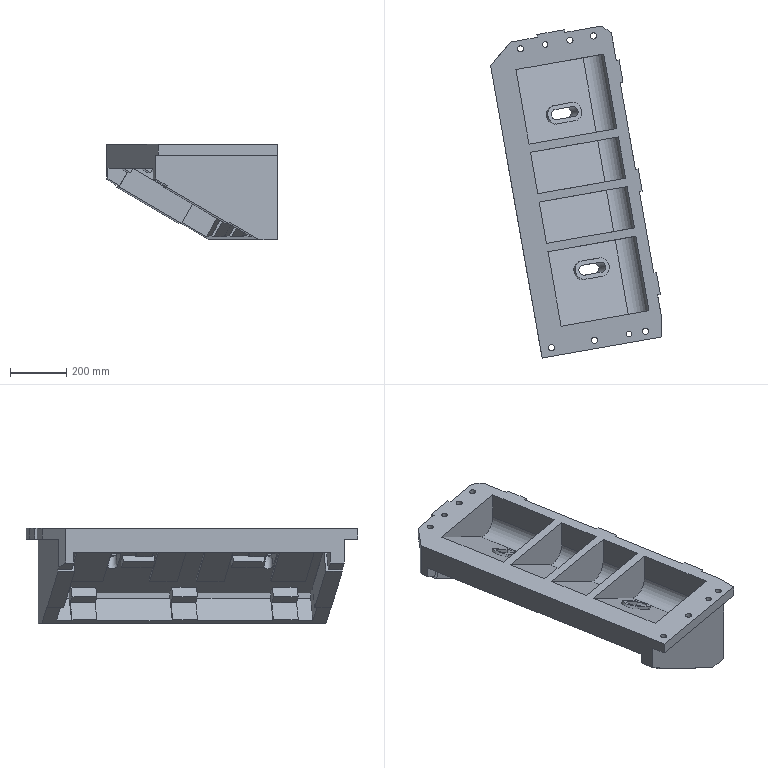Part | NX | features solid 2 | 1 solid | 180 faces | box 609.849 x 1185 x 339.158 mm | volume 53245270 mm3 | plane 154 | cylinder 26 | commonest cylinder face diameters 22 x6 32 x6 36 x4 66 x4 100 x4 20 x2